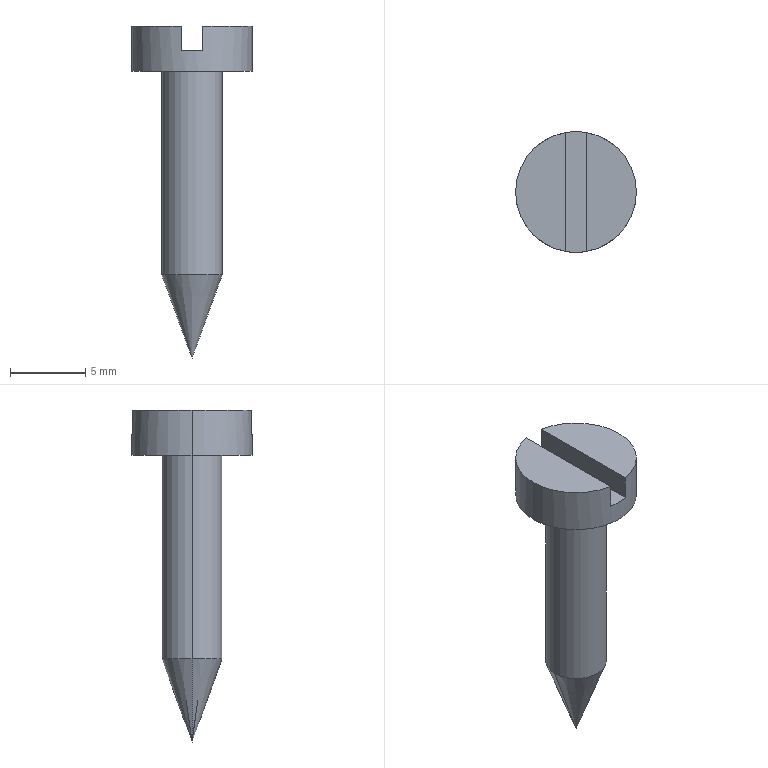Part | SolidWorks | features ICE 2, Extrusion 1, RevCut 1 | 1 solid | 12 faces | box 8 x 8 x 22 mm | volume 325.653 mm3 | plane 6 | cylinder 4 | cone 2 | commonest cylinder face diameters 4 x2 8 x2
STEP:
#1=CARTESIAN_POINT('',(0.,0.,-19.));
#2=VERTEX_POINT('',#1);
#3=CARTESIAN_POINT('',(2.,0.,-13.5));
#4=VERTEX_POINT('',#3);
#5=CARTESIAN_POINT('',(0.,0.,-19.));
#6=DIRECTION('',(0.3417,0.,0.9398));
#7=VECTOR('',#6,1000.);
#8=LINE('',#5,#7);
#9=EDGE_CURVE('',#2,#4,#8,.T.);
#10=ORIENTED_EDGE('',*,*,#9,.F.);
#11=CARTESIAN_POINT('',(-2.,0.,-13.5));
#12=VERTEX_POINT('',#11);
#13=CARTESIAN_POINT('',(0.,0.,-19.));
#14=DIRECTION('',(-0.3417,0.,0.9398));
#15=VECTOR('',#14,1000.);
#16=LINE('',#13,#15);
#17=EDGE_CURVE('',#2,#12,#16,.T.);
#18=ORIENTED_EDGE('',*,*,#17,.T.);
#19=CARTESIAN_POINT('',(0.,0.,-13.5));
#20=DIRECTION('',(0.,0.,-1.));
#21=DIRECTION('',(-1.,0.,0.));
#22=AXIS2_PLACEMENT_3D('',#19,#20,#21);
#23=CIRCLE('',#22,2.);
#24=EDGE_CURVE('',#12,#4,#23,.T.);
#25=ORIENTED_EDGE('',*,*,#24,.T.);
#26=EDGE_LOOP('',(#10,#18,#25));
#27=FACE_OUTER_BOUND('',#26,.T.);
#28=CARTESIAN_POINT('',(0.,0.,981.));
#29=DIRECTION('',(0.,0.,1.));
#30=DIRECTION('',(1.,0.,0.));
#31=AXIS2_PLACEMENT_3D('',#28,#29,#30);
#32=CONICAL_SURFACE('',#31,363.636,0.3488);
#33=ADVANCED_FACE('',(#27),#32,.T.);
#34=CARTESIAN_POINT('',(4.,0.,3.));
#35=VERTEX_POINT('',#34);
#36=CARTESIAN_POINT('',(0.7,3.938,3.));
#37=VERTEX_POINT('',#36);
#38=CARTESIAN_POINT('',(0.,0.,3.));
#39=DIRECTION('',(0.,0.,1.));
#40=DIRECTION('',(1.,0.,0.));
#41=AXIS2_PLACEMENT_3D('',#38,#39,#40);
#42=CIRCLE('',#41,4.);
#43=EDGE_CURVE('',#35,#37,#42,.T.);
#44=ORIENTED_EDGE('',*,*,#43,.F.);
#45=CARTESIAN_POINT('',(4.,0.,0.));
#46=VERTEX_POINT('',#45);
#47=CARTESIAN_POINT('',(4.,0.,3.));
#48=DIRECTION('',(0.,0.,-1.));
#49=VECTOR('',#48,1000.);
#50=LINE('',#47,#49);
#51=EDGE_CURVE('',#35,#46,#50,.T.);
#52=ORIENTED_EDGE('',*,*,#51,.T.);
#53=CARTESIAN_POINT('',(-4.,0.,0.));
#54=VERTEX_POINT('',#53);
#55=CARTESIAN_POINT('',(0.,0.,0.));
#56=DIRECTION('',(0.,0.,1.));
#57=DIRECTION('',(1.,0.,0.));
#58=AXIS2_PLACEMENT_3D('',#55,#56,#57);
#59=CIRCLE('',#58,4.);
#60=EDGE_CURVE('',#46,#54,#59,.T.);
#61=ORIENTED_EDGE('',*,*,#60,.T.);
#62=CARTESIAN_POINT('',(-4.,0.,3.));
#63=VERTEX_POINT('',#62);
#64=CARTESIAN_POINT('',(-4.,0.,3.));
#65=DIRECTION('',(0.,0.,-1.));
#66=VECTOR('',#65,1000.);
#67=LINE('',#64,#66);
#68=EDGE_CURVE('',#63,#54,#67,.T.);
#69=ORIENTED_EDGE('',*,*,#68,.F.);
#70=CARTESIAN_POINT('',(-0.7,3.938,3.));
#71=VERTEX_POINT('',#70);
#72=CARTESIAN_POINT('',(0.,0.,3.));
#73=DIRECTION('',(0.,0.,1.));
#74=DIRECTION('',(1.,0.,0.));
#75=AXIS2_PLACEMENT_3D('',#72,#73,#74);
#76=CIRCLE('',#75,4.);
#77=EDGE_CURVE('',#71,#63,#76,.T.);
#78=ORIENTED_EDGE('',*,*,#77,.F.);
#79=CARTESIAN_POINT('',(-0.7,3.938,1.4));
#80=VERTEX_POINT('',#79);
#81=CARTESIAN_POINT('',(-0.7,3.938,3.));
#82=DIRECTION('',(0.,0.,-1.));
#83=VECTOR('',#82,1000.);
#84=LINE('',#81,#83);
#85=EDGE_CURVE('',#71,#80,#84,.T.);
#86=ORIENTED_EDGE('',*,*,#85,.T.);
#87=CARTESIAN_POINT('',(0.7,3.938,1.4));
#88=VERTEX_POINT('',#87);
#89=CARTESIAN_POINT('',(0.,0.,1.4));
#90=DIRECTION('',(0.,0.,-1.));
#91=DIRECTION('',(-1.,0.,0.));
#92=AXIS2_PLACEMENT_3D('',#89,#90,#91);
#93=CIRCLE('',#92,4.);
#94=EDGE_CURVE('',#80,#88,#93,.T.);
#95=ORIENTED_EDGE('',*,*,#94,.T.);
#96=CARTESIAN_POINT('',(0.7,3.938,3.));
#97=DIRECTION('',(0.,0.,1.));
#98=VECTOR('',#97,1000.);
#99=LINE('',#96,#98);
#100=EDGE_CURVE('',#88,#37,#99,.T.);
#101=ORIENTED_EDGE('',*,*,#100,.T.);
#102=EDGE_LOOP('',(#44,#52,#61,#69,#78,#86,#95,#101));
#103=FACE_OUTER_BOUND('',#102,.T.);
#104=CARTESIAN_POINT('',(0.,0.,3.));
#105=DIRECTION('',(0.,0.,-1.));
#106=DIRECTION('',(-1.,0.,0.));
#107=AXIS2_PLACEMENT_3D('',#104,#105,#106);
#108=CYLINDRICAL_SURFACE('',#107,4.);
#109=ADVANCED_FACE('',(#103),#108,.T.);
#110=ORIENTED_EDGE('',*,*,#24,.F.);
#111=CARTESIAN_POINT('',(-2.,0.,0.));
#112=VERTEX_POINT('',#111);
#113=CARTESIAN_POINT('',(-2.,0.,-19.));
#114=DIRECTION('',(0.,0.,1.));
#115=VECTOR('',#114,1000.);
#116=LINE('',#113,#115);
#117=EDGE_CURVE('',#12,#112,#116,.T.);
#118=ORIENTED_EDGE('',*,*,#117,.T.);
#119=CARTESIAN_POINT('',(2.,0.,0.));
#120=VERTEX_POINT('',#119);
#121=CARTESIAN_POINT('',(0.,0.,0.));
#122=DIRECTION('',(0.,0.,-1.));
#123=DIRECTION('',(-1.,0.,0.));
#124=AXIS2_PLACEMENT_3D('',#121,#122,#123);
#125=CIRCLE('',#124,2.);
#126=EDGE_CURVE('',#112,#120,#125,.T.);
#127=ORIENTED_EDGE('',*,*,#126,.T.);
#128=CARTESIAN_POINT('',(2.,0.,-19.));
#129=DIRECTION('',(0.,0.,1.));
#130=VECTOR('',#129,1000.);
#131=LINE('',#128,#130);
#132=EDGE_CURVE('',#4,#120,#131,.T.);
#133=ORIENTED_EDGE('',*,*,#132,.F.);
#134=EDGE_LOOP('',(#110,#118,#127,#133));
#135=FACE_OUTER_BOUND('',#134,.T.);
#136=CARTESIAN_POINT('',(0.,0.,-19.));
#137=DIRECTION('',(0.,0.,1.));
#138=DIRECTION('',(1.,0.,0.));
#139=AXIS2_PLACEMENT_3D('',#136,#137,#138);
#140=CYLINDRICAL_SURFACE('',#139,2.);
#141=ADVANCED_FACE('',(#135),#140,.T.);
#142=ORIENTED_EDGE('',*,*,#117,.F.);
#143=CARTESIAN_POINT('',(0.,0.,-13.5));
#144=DIRECTION('',(0.,0.,-1.));
#145=DIRECTION('',(-1.,0.,0.));
#146=AXIS2_PLACEMENT_3D('',#143,#144,#145);
#147=CIRCLE('',#146,2.);
#148=EDGE_CURVE('',#4,#12,#147,.T.);
#149=ORIENTED_EDGE('',*,*,#148,.F.);
#150=ORIENTED_EDGE('',*,*,#132,.T.);
#151=CARTESIAN_POINT('',(0.,0.,0.));
#152=DIRECTION('',(0.,0.,-1.));
#153=DIRECTION('',(-1.,0.,0.));
#154=AXIS2_PLACEMENT_3D('',#151,#152,#153);
#155=CIRCLE('',#154,2.);
#156=EDGE_CURVE('',#120,#112,#155,.T.);
#157=ORIENTED_EDGE('',*,*,#156,.T.);
#158=EDGE_LOOP('',(#142,#149,#150,#157));
#159=FACE_OUTER_BOUND('',#158,.T.);
#160=CARTESIAN_POINT('',(0.,0.,-19.));
#161=DIRECTION('',(0.,0.,1.));
#162=DIRECTION('',(1.,0.,0.));
#163=AXIS2_PLACEMENT_3D('',#160,#161,#162);
#164=CYLINDRICAL_SURFACE('',#163,2.);
#165=ADVANCED_FACE('',(#159),#164,.T.);
#166=CARTESIAN_POINT('',(-0.7,-3.938,3.));
#167=VERTEX_POINT('',#166);
#168=CARTESIAN_POINT('',(-0.7,0.,3.));
#169=DIRECTION('',(0.,-1.,0.));
#170=VECTOR('',#169,1000.);
#171=LINE('',#168,#170);
#172=EDGE_CURVE('',#71,#167,#171,.T.);
#173=ORIENTED_EDGE('',*,*,#172,.F.);
#174=ORIENTED_EDGE('',*,*,#77,.T.);
#175=CARTESIAN_POINT('',(0.,0.,3.));
#176=DIRECTION('',(0.,0.,1.));
#177=DIRECTION('',(1.,0.,0.));
#178=AXIS2_PLACEMENT_3D('',#175,#176,#177);
#179=CIRCLE('',#178,4.);
#180=EDGE_CURVE('',#63,#167,#179,.T.);
#181=ORIENTED_EDGE('',*,*,#180,.T.);
#182=EDGE_LOOP('',(#173,#174,#181));
#183=FACE_OUTER_BOUND('',#182,.T.);
#184=CARTESIAN_POINT('',(0.,0.,3.));
#185=DIRECTION('',(0.,0.,1.));
#186=DIRECTION('',(1.,0.,0.));
#187=AXIS2_PLACEMENT_3D('',#184,#185,#186);
#188=PLANE('',#187);
#189=ADVANCED_FACE('',(#183),#188,.T.);
#190=ORIENTED_EDGE('',*,*,#51,.F.);
#191=CARTESIAN_POINT('',(0.7,-3.938,3.));
#192=VERTEX_POINT('',#191);
#193=CARTESIAN_POINT('',(0.,0.,3.));
#194=DIRECTION('',(0.,0.,1.));
#195=DIRECTION('',(1.,0.,0.));
#196=AXIS2_PLACEMENT_3D('',#193,#194,#195);
#197=CIRCLE('',#196,4.);
#198=EDGE_CURVE('',#192,#35,#197,.T.);
#199=ORIENTED_EDGE('',*,*,#198,.F.);
#200=CARTESIAN_POINT('',(0.7,-3.938,1.4));
#201=VERTEX_POINT('',#200);
#202=CARTESIAN_POINT('',(0.7,-3.938,3.));
#203=DIRECTION('',(0.,0.,-1.));
#204=VECTOR('',#203,1000.);
#205=LINE('',#202,#204);
#206=EDGE_CURVE('',#192,#201,#205,.T.);
#207=ORIENTED_EDGE('',*,*,#206,.T.);
#208=CARTESIAN_POINT('',(-0.7,-3.938,1.4));
#209=VERTEX_POINT('',#208);
#210=CARTESIAN_POINT('',(0.,0.,1.4));
#211=DIRECTION('',(0.,0.,-1.));
#212=DIRECTION('',(-1.,0.,0.));
#213=AXIS2_PLACEMENT_3D('',#210,#211,#212);
#214=CIRCLE('',#213,4.);
#215=EDGE_CURVE('',#201,#209,#214,.T.);
#216=ORIENTED_EDGE('',*,*,#215,.T.);
#217=CARTESIAN_POINT('',(-0.7,-3.938,3.));
#218=DIRECTION('',(0.,0.,1.));
#219=VECTOR('',#218,1000.);
#220=LINE('',#217,#219);
#221=EDGE_CURVE('',#209,#167,#220,.T.);
#222=ORIENTED_EDGE('',*,*,#221,.T.);
#223=ORIENTED_EDGE('',*,*,#180,.F.);
#224=ORIENTED_EDGE('',*,*,#68,.T.);
#225=CARTESIAN_POINT('',(0.,0.,0.));
#226=DIRECTION('',(0.,0.,1.));
#227=DIRECTION('',(1.,0.,0.));
#228=AXIS2_PLACEMENT_3D('',#225,#226,#227);
#229=CIRCLE('',#228,4.);
#230=EDGE_CURVE('',#54,#46,#229,.T.);
#231=ORIENTED_EDGE('',*,*,#230,.T.);
#232=EDGE_LOOP('',(#190,#199,#207,#216,#222,#223,#224,#231));
#233=FACE_OUTER_BOUND('',#232,.T.);
#234=CARTESIAN_POINT('',(0.,0.,3.));
#235=DIRECTION('',(0.,0.,-1.));
#236=DIRECTION('',(-1.,0.,0.));
#237=AXIS2_PLACEMENT_3D('',#234,#235,#236);
#238=CYLINDRICAL_SURFACE('',#237,4.);
#239=ADVANCED_FACE('',(#233),#238,.T.);
#240=CARTESIAN_POINT('',(0.7,0.,3.));
#241=DIRECTION('',(0.,1.,0.));
#242=VECTOR('',#241,1000.);
#243=LINE('',#240,#242);
#244=EDGE_CURVE('',#192,#37,#243,.T.);
#245=ORIENTED_EDGE('',*,*,#244,.F.);
#246=ORIENTED_EDGE('',*,*,#198,.T.);
#247=ORIENTED_EDGE('',*,*,#43,.T.);
#248=EDGE_LOOP('',(#245,#246,#247));
#249=FACE_OUTER_BOUND('',#248,.T.);
#250=CARTESIAN_POINT('',(0.,0.,3.));
#251=DIRECTION('',(0.,0.,1.));
#252=DIRECTION('',(1.,0.,0.));
#253=AXIS2_PLACEMENT_3D('',#250,#251,#252);
#254=PLANE('',#253);
#255=ADVANCED_FACE('',(#249),#254,.T.);
#256=ORIENTED_EDGE('',*,*,#156,.F.);
#257=ORIENTED_EDGE('',*,*,#126,.F.);
#258=EDGE_LOOP('',(#256,#257));
#259=FACE_BOUND('',#258,.T.);
#260=ORIENTED_EDGE('',*,*,#230,.F.);
#261=ORIENTED_EDGE('',*,*,#60,.F.);
#262=EDGE_LOOP('',(#260,#261));
#263=FACE_OUTER_BOUND('',#262,.T.);
#264=CARTESIAN_POINT('',(0.,0.,0.));
#265=DIRECTION('',(0.,0.,1.));
#266=DIRECTION('',(1.,0.,0.));
#267=AXIS2_PLACEMENT_3D('',#264,#265,#266);
#268=PLANE('',#267);
#269=ADVANCED_FACE('',(#259,#263),#268,.F.);
#270=CARTESIAN_POINT('',(-0.7,4.828,1.4));
#271=DIRECTION('',(0.,-1.,0.));
#272=VECTOR('',#271,1000.);
#273=LINE('',#270,#272);
#274=EDGE_CURVE('',#80,#209,#273,.T.);
#275=ORIENTED_EDGE('',*,*,#274,.T.);
#276=ORIENTED_EDGE('',*,*,#215,.F.);
#277=CARTESIAN_POINT('',(0.7,4.828,1.4));
#278=DIRECTION('',(0.,1.,0.));
#279=VECTOR('',#278,1000.);
#280=LINE('',#277,#279);
#281=EDGE_CURVE('',#201,#88,#280,.T.);
#282=ORIENTED_EDGE('',*,*,#281,.T.);
#283=ORIENTED_EDGE('',*,*,#94,.F.);
#284=EDGE_LOOP('',(#275,#276,#282,#283));
#285=FACE_OUTER_BOUND('',#284,.T.);
#286=CARTESIAN_POINT('',(0.,0.,1.4));
#287=DIRECTION('',(0.,0.,-1.));
#288=DIRECTION('',(-1.,0.,0.));
#289=AXIS2_PLACEMENT_3D('',#286,#287,#288);
#290=PLANE('',#289);
#291=ADVANCED_FACE('',(#285),#290,.F.);
#292=ORIENTED_EDGE('',*,*,#172,.T.);
#293=ORIENTED_EDGE('',*,*,#221,.F.);
#294=ORIENTED_EDGE('',*,*,#274,.F.);
#295=ORIENTED_EDGE('',*,*,#85,.F.);
#296=EDGE_LOOP('',(#292,#293,#294,#295));
#297=FACE_OUTER_BOUND('',#296,.T.);
#298=CARTESIAN_POINT('',(-0.7,4.828,1.4));
#299=DIRECTION('',(-1.,0.,0.));
#300=DIRECTION('',(0.,-1.,0.));
#301=AXIS2_PLACEMENT_3D('',#298,#299,#300);
#302=PLANE('',#301);
#303=ADVANCED_FACE('',(#297),#302,.F.);
#304=ORIENTED_EDGE('',*,*,#244,.T.);
#305=ORIENTED_EDGE('',*,*,#100,.F.);
#306=ORIENTED_EDGE('',*,*,#281,.F.);
#307=ORIENTED_EDGE('',*,*,#206,.F.);
#308=EDGE_LOOP('',(#304,#305,#306,#307));
#309=FACE_OUTER_BOUND('',#308,.T.);
#310=CARTESIAN_POINT('',(0.7,4.828,1.4));
#311=DIRECTION('',(1.,0.,0.));
#312=DIRECTION('',(0.,1.,0.));
#313=AXIS2_PLACEMENT_3D('',#310,#311,#312);
#314=PLANE('',#313);
#315=ADVANCED_FACE('',(#309),#314,.F.);
#316=ORIENTED_EDGE('',*,*,#17,.F.);
#317=ORIENTED_EDGE('',*,*,#9,.T.);
#318=ORIENTED_EDGE('',*,*,#148,.T.);
#319=EDGE_LOOP('',(#316,#317,#318));
#320=FACE_OUTER_BOUND('',#319,.T.);
#321=CARTESIAN_POINT('',(0.,0.,981.));
#322=DIRECTION('',(0.,0.,1.));
#323=DIRECTION('',(1.,0.,0.));
#324=AXIS2_PLACEMENT_3D('',#321,#322,#323);
#325=CONICAL_SURFACE('',#324,363.636,0.3488);
#326=ADVANCED_FACE('',(#320),#325,.T.);
#327=CLOSED_SHELL('',(#33,#109,#141,#165,#189,#239,#255,#269,#291,#303,#315,#326));
#328=MANIFOLD_SOLID_BREP('',#327);
#329=CARTESIAN_POINT('',(0.,0.,0.));
#330=DIRECTION('',(0.,0.,1.));
#331=DIRECTION('',(1.,0.,0.));
#332=AXIS2_PLACEMENT_3D('',#329,#330,#331);
#333=(LENGTH_UNIT()NAMED_UNIT(*)SI_UNIT(.MILLI.,.METRE.));
#334=UNCERTAINTY_MEASURE_WITH_UNIT(LENGTH_MEASURE(0.00001),#333,'','');
#335=(NAMED_UNIT(*)PLANE_ANGLE_UNIT()SI_UNIT($,.RADIAN.));
#336=(NAMED_UNIT(*)SI_UNIT($,.STERADIAN.)SOLID_ANGLE_UNIT());
#337=(GEOMETRIC_REPRESENTATION_CONTEXT(3)GLOBAL_UNCERTAINTY_ASSIGNED_CONTEXT((#334))GLOBAL_UNIT_ASSIGNED_CONTEXT((#333,#335,#336))REPRESENTATION_CONTEXT('',''));
#338=ADVANCED_BREP_SHAPE_REPRESENTATION('',(#328,#332),#337);